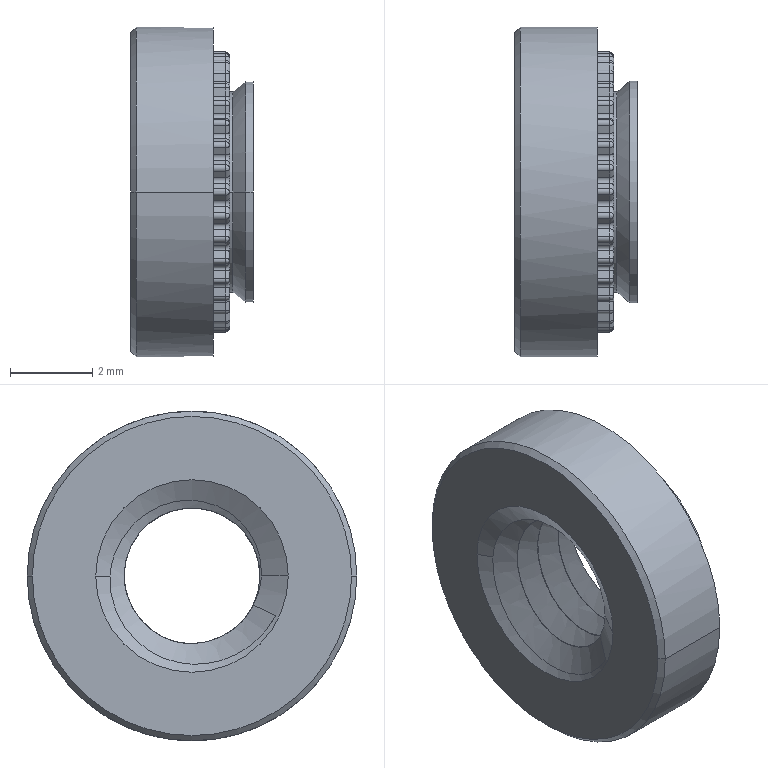Part | NX | features solid 2 | 1 solid | 316 faces | box 2.97 x 8 x 8 mm | volume 88.842 mm3 | cylinder 156 | plane 76 | torus 36 | sphere 36 | cone 8 | spline 4 | commonest cylinder face diameters 0.2 x144 3.3 x6 4.86 x2 5.38 x2 8 x2